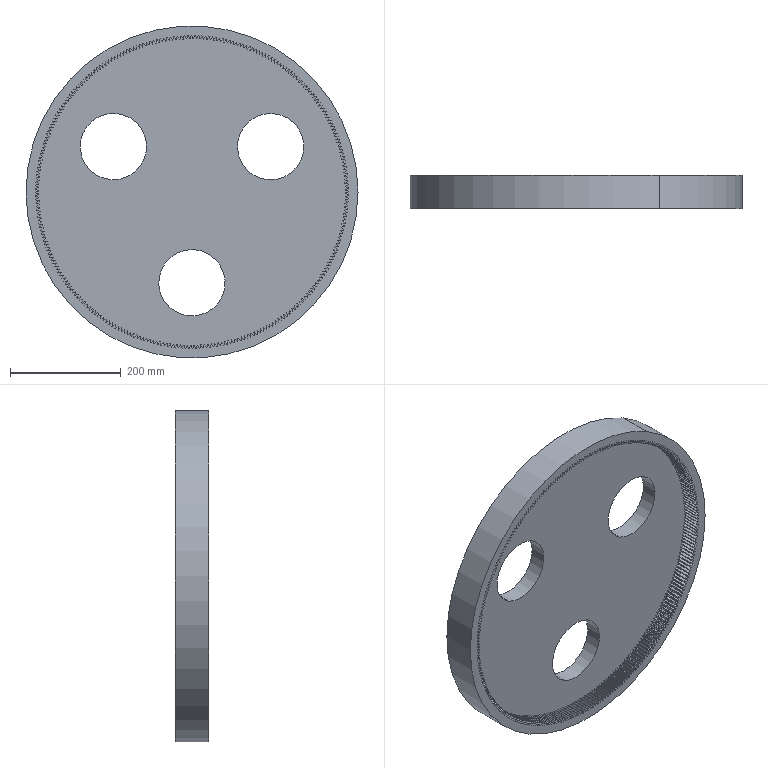Part | STEP file | 2026.6.15-Main Assembly图.sldasm-Part-16 | 1 solid | 1131 faces | box 600 x 60 x 600 mm | volume 8563551 mm3 | cylinder 568 | spline 560 | plane 3 | commonest cylinder face diameters 553.932 x280 565 x280 120 x6 600 x2